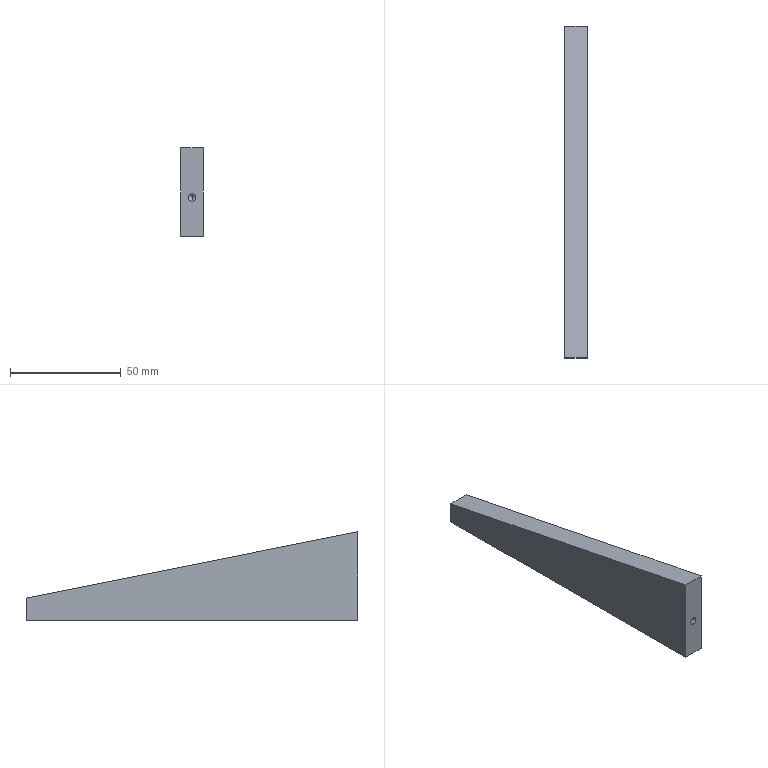Part | SolidWorks | features HoleWzd 2, Chamfer 1, Extrusion 1 | 1 solid | 22 faces | box 10 x 150 x 40 mm | volume 37104 mm3 | cylinder 8 | cone 8 | plane 6 | commonest cylinder face diameters 3.3 x8
STEP:
#1=CARTESIAN_POINT('',(0.,-60.,19.15));
#2=VERTEX_POINT('',#1);
#3=CARTESIAN_POINT('',(0.,-60.,15.85));
#4=VERTEX_POINT('',#3);
#5=CARTESIAN_POINT('',(0.,-60.,17.5));
#6=DIRECTION('',(0.,-1.,0.));
#7=DIRECTION('',(0.,0.,-1.));
#8=AXIS2_PLACEMENT_3D('',#5,#6,#7);
#9=CIRCLE('',#8,1.65);
#10=EDGE_CURVE('',#2,#4,#9,.T.);
#11=ORIENTED_EDGE('',*,*,#10,.F.);
#12=CARTESIAN_POINT('',(0.,-75.,19.15));
#13=VERTEX_POINT('',#12);
#14=CARTESIAN_POINT('',(0.,-75.,19.15));
#15=DIRECTION('',(0.,-1.,0.));
#16=VECTOR('',#15,1000.);
#17=LINE('',#14,#16);
#18=EDGE_CURVE('',#2,#13,#17,.T.);
#19=ORIENTED_EDGE('',*,*,#18,.T.);
#20=CARTESIAN_POINT('',(0.,-75.,15.85));
#21=VERTEX_POINT('',#20);
#22=CARTESIAN_POINT('',(0.,-75.,17.5));
#23=DIRECTION('',(0.,-1.,0.));
#24=DIRECTION('',(0.,0.,-1.));
#25=AXIS2_PLACEMENT_3D('',#22,#23,#24);
#26=CIRCLE('',#25,1.65);
#27=EDGE_CURVE('',#13,#21,#26,.T.);
#28=ORIENTED_EDGE('',*,*,#27,.T.);
#29=CARTESIAN_POINT('',(0.,-75.,15.85));
#30=DIRECTION('',(0.,-1.,0.));
#31=VECTOR('',#30,1000.);
#32=LINE('',#29,#31);
#33=EDGE_CURVE('',#4,#21,#32,.T.);
#34=ORIENTED_EDGE('',*,*,#33,.F.);
#35=EDGE_LOOP('',(#11,#19,#28,#34));
#36=FACE_OUTER_BOUND('',#35,.T.);
#37=CARTESIAN_POINT('',(0.,-75.,17.5));
#38=DIRECTION('',(0.,-1.,0.));
#39=DIRECTION('',(0.,0.,-1.));
#40=AXIS2_PLACEMENT_3D('',#37,#38,#39);
#41=CYLINDRICAL_SURFACE('',#40,1.65);
#42=ADVANCED_FACE('',(#36),#41,.F.);
#43=CARTESIAN_POINT('',(0.,-59.009,17.5));
#44=VERTEX_POINT('',#43);
#45=CARTESIAN_POINT('',(0.,-60.,15.85));
#46=DIRECTION('',(0.,-0.515,-0.8572));
#47=VECTOR('',#46,1000.);
#48=LINE('',#45,#47);
#49=EDGE_CURVE('',#44,#4,#48,.T.);
#50=ORIENTED_EDGE('',*,*,#49,.F.);
#51=CARTESIAN_POINT('',(0.,-60.,19.15));
#52=DIRECTION('',(0.,-0.515,0.8572));
#53=VECTOR('',#52,1000.);
#54=LINE('',#51,#53);
#55=EDGE_CURVE('',#44,#2,#54,.T.);
#56=ORIENTED_EDGE('',*,*,#55,.T.);
#57=ORIENTED_EDGE('',*,*,#10,.T.);
#58=EDGE_LOOP('',(#50,#56,#57));
#59=FACE_OUTER_BOUND('',#58,.T.);
#60=CARTESIAN_POINT('',(0.,-60.,17.5));
#61=DIRECTION('',(0.,-1.,0.));
#62=DIRECTION('',(0.,0.,-1.));
#63=AXIS2_PLACEMENT_3D('',#60,#61,#62);
#64=CONICAL_SURFACE('',#63,1.65,1.03);
#65=ADVANCED_FACE('',(#59),#64,.F.);
#66=CARTESIAN_POINT('',(1.65,50.,10.));
#67=VERTEX_POINT('',#66);
#68=CARTESIAN_POINT('',(-1.65,50.,10.));
#69=VERTEX_POINT('',#68);
#70=CARTESIAN_POINT('',(0.,50.,10.));
#71=DIRECTION('',(0.,0.,-1.));
#72=DIRECTION('',(-1.,0.,0.));
#73=AXIS2_PLACEMENT_3D('',#70,#71,#72);
#74=CIRCLE('',#73,1.65);
#75=EDGE_CURVE('',#67,#69,#74,.T.);
#76=ORIENTED_EDGE('',*,*,#75,.F.);
#77=CARTESIAN_POINT('',(1.65,50.,0.));
#78=VERTEX_POINT('',#77);
#79=CARTESIAN_POINT('',(1.65,50.,0.));
#80=DIRECTION('',(0.,0.,-1.));
#81=VECTOR('',#80,1000.);
#82=LINE('',#79,#81);
#83=EDGE_CURVE('',#67,#78,#82,.T.);
#84=ORIENTED_EDGE('',*,*,#83,.T.);
#85=CARTESIAN_POINT('',(-1.65,50.,0.));
#86=VERTEX_POINT('',#85);
#87=CARTESIAN_POINT('',(0.,50.,0.));
#88=DIRECTION('',(0.,0.,-1.));
#89=DIRECTION('',(-1.,0.,0.));
#90=AXIS2_PLACEMENT_3D('',#87,#88,#89);
#91=CIRCLE('',#90,1.65);
#92=EDGE_CURVE('',#78,#86,#91,.T.);
#93=ORIENTED_EDGE('',*,*,#92,.T.);
#94=CARTESIAN_POINT('',(-1.65,50.,0.));
#95=DIRECTION('',(0.,0.,-1.));
#96=VECTOR('',#95,1000.);
#97=LINE('',#94,#96);
#98=EDGE_CURVE('',#69,#86,#97,.T.);
#99=ORIENTED_EDGE('',*,*,#98,.F.);
#100=EDGE_LOOP('',(#76,#84,#93,#99));
#101=FACE_OUTER_BOUND('',#100,.T.);
#102=CARTESIAN_POINT('',(0.,50.,0.));
#103=DIRECTION('',(0.,0.,-1.));
#104=DIRECTION('',(-1.,0.,0.));
#105=AXIS2_PLACEMENT_3D('',#102,#103,#104);
#106=CYLINDRICAL_SURFACE('',#105,1.65);
#107=ADVANCED_FACE('',(#101),#106,.F.);
#108=CARTESIAN_POINT('',(0.,50.,10.991));
#109=VERTEX_POINT('',#108);
#110=CARTESIAN_POINT('',(-1.65,50.,10.));
#111=DIRECTION('',(-0.8572,0.,-0.515));
#112=VECTOR('',#111,1000.);
#113=LINE('',#110,#112);
#114=EDGE_CURVE('',#109,#69,#113,.T.);
#115=ORIENTED_EDGE('',*,*,#114,.F.);
#116=CARTESIAN_POINT('',(1.65,50.,10.));
#117=DIRECTION('',(0.8572,0.,-0.515));
#118=VECTOR('',#117,1000.);
#119=LINE('',#116,#118);
#120=EDGE_CURVE('',#109,#67,#119,.T.);
#121=ORIENTED_EDGE('',*,*,#120,.T.);
#122=ORIENTED_EDGE('',*,*,#75,.T.);
#123=EDGE_LOOP('',(#115,#121,#122));
#124=FACE_OUTER_BOUND('',#123,.T.);
#125=CARTESIAN_POINT('',(0.,50.,10.));
#126=DIRECTION('',(0.,0.,-1.));
#127=DIRECTION('',(-1.,0.,0.));
#128=AXIS2_PLACEMENT_3D('',#125,#126,#127);
#129=CONICAL_SURFACE('',#128,1.65,1.03);
#130=ADVANCED_FACE('',(#124),#129,.F.);
#131=CARTESIAN_POINT('',(1.65,0.,10.));
#132=VERTEX_POINT('',#131);
#133=CARTESIAN_POINT('',(-1.65,0.,10.));
#134=VERTEX_POINT('',#133);
#135=CARTESIAN_POINT('',(0.,0.,10.));
#136=DIRECTION('',(0.,0.,-1.));
#137=DIRECTION('',(-1.,0.,0.));
#138=AXIS2_PLACEMENT_3D('',#135,#136,#137);
#139=CIRCLE('',#138,1.65);
#140=EDGE_CURVE('',#132,#134,#139,.T.);
#141=ORIENTED_EDGE('',*,*,#140,.F.);
#142=CARTESIAN_POINT('',(1.65,0.,0.));
#143=VERTEX_POINT('',#142);
#144=CARTESIAN_POINT('',(1.65,0.,0.));
#145=DIRECTION('',(0.,0.,-1.));
#146=VECTOR('',#145,1000.);
#147=LINE('',#144,#146);
#148=EDGE_CURVE('',#132,#143,#147,.T.);
#149=ORIENTED_EDGE('',*,*,#148,.T.);
#150=CARTESIAN_POINT('',(-1.65,0.,0.));
#151=VERTEX_POINT('',#150);
#152=CARTESIAN_POINT('',(0.,0.,0.));
#153=DIRECTION('',(0.,0.,-1.));
#154=DIRECTION('',(-1.,0.,0.));
#155=AXIS2_PLACEMENT_3D('',#152,#153,#154);
#156=CIRCLE('',#155,1.65);
#157=EDGE_CURVE('',#143,#151,#156,.T.);
#158=ORIENTED_EDGE('',*,*,#157,.T.);
#159=CARTESIAN_POINT('',(-1.65,0.,0.));
#160=DIRECTION('',(0.,0.,-1.));
#161=VECTOR('',#160,1000.);
#162=LINE('',#159,#161);
#163=EDGE_CURVE('',#134,#151,#162,.T.);
#164=ORIENTED_EDGE('',*,*,#163,.F.);
#165=EDGE_LOOP('',(#141,#149,#158,#164));
#166=FACE_OUTER_BOUND('',#165,.T.);
#167=CARTESIAN_POINT('',(0.,0.,0.));
#168=DIRECTION('',(0.,0.,-1.));
#169=DIRECTION('',(-1.,0.,0.));
#170=AXIS2_PLACEMENT_3D('',#167,#168,#169);
#171=CYLINDRICAL_SURFACE('',#170,1.65);
#172=ADVANCED_FACE('',(#166),#171,.F.);
#173=CARTESIAN_POINT('',(0.,0.,10.991));
#174=VERTEX_POINT('',#173);
#175=CARTESIAN_POINT('',(-1.65,0.,10.));
#176=DIRECTION('',(-0.8572,0.,-0.515));
#177=VECTOR('',#176,1000.);
#178=LINE('',#175,#177);
#179=EDGE_CURVE('',#174,#134,#178,.T.);
#180=ORIENTED_EDGE('',*,*,#179,.F.);
#181=CARTESIAN_POINT('',(1.65,0.,10.));
#182=DIRECTION('',(0.8572,0.,-0.515));
#183=VECTOR('',#182,1000.);
#184=LINE('',#181,#183);
#185=EDGE_CURVE('',#174,#132,#184,.T.);
#186=ORIENTED_EDGE('',*,*,#185,.T.);
#187=ORIENTED_EDGE('',*,*,#140,.T.);
#188=EDGE_LOOP('',(#180,#186,#187));
#189=FACE_OUTER_BOUND('',#188,.T.);
#190=CARTESIAN_POINT('',(0.,0.,10.));
#191=DIRECTION('',(0.,0.,-1.));
#192=DIRECTION('',(-1.,0.,0.));
#193=AXIS2_PLACEMENT_3D('',#190,#191,#192);
#194=CONICAL_SURFACE('',#193,1.65,1.03);
#195=ADVANCED_FACE('',(#189),#194,.F.);
#196=CARTESIAN_POINT('',(1.65,-50.,10.));
#197=VERTEX_POINT('',#196);
#198=CARTESIAN_POINT('',(-1.65,-50.,10.));
#199=VERTEX_POINT('',#198);
#200=CARTESIAN_POINT('',(0.,-50.,10.));
#201=DIRECTION('',(0.,0.,-1.));
#202=DIRECTION('',(-1.,0.,0.));
#203=AXIS2_PLACEMENT_3D('',#200,#201,#202);
#204=CIRCLE('',#203,1.65);
#205=EDGE_CURVE('',#197,#199,#204,.T.);
#206=ORIENTED_EDGE('',*,*,#205,.F.);
#207=CARTESIAN_POINT('',(1.65,-50.,0.));
#208=VERTEX_POINT('',#207);
#209=CARTESIAN_POINT('',(1.65,-50.,0.));
#210=DIRECTION('',(0.,0.,-1.));
#211=VECTOR('',#210,1000.);
#212=LINE('',#209,#211);
#213=EDGE_CURVE('',#197,#208,#212,.T.);
#214=ORIENTED_EDGE('',*,*,#213,.T.);
#215=CARTESIAN_POINT('',(-1.65,-50.,0.));
#216=VERTEX_POINT('',#215);
#217=CARTESIAN_POINT('',(0.,-50.,0.));
#218=DIRECTION('',(0.,0.,-1.));
#219=DIRECTION('',(-1.,0.,0.));
#220=AXIS2_PLACEMENT_3D('',#217,#218,#219);
#221=CIRCLE('',#220,1.65);
#222=EDGE_CURVE('',#208,#216,#221,.T.);
#223=ORIENTED_EDGE('',*,*,#222,.T.);
#224=CARTESIAN_POINT('',(-1.65,-50.,0.));
#225=DIRECTION('',(0.,0.,-1.));
#226=VECTOR('',#225,1000.);
#227=LINE('',#224,#226);
#228=EDGE_CURVE('',#199,#216,#227,.T.);
#229=ORIENTED_EDGE('',*,*,#228,.F.);
#230=EDGE_LOOP('',(#206,#214,#223,#229));
#231=FACE_OUTER_BOUND('',#230,.T.);
#232=CARTESIAN_POINT('',(0.,-50.,0.));
#233=DIRECTION('',(0.,0.,-1.));
#234=DIRECTION('',(-1.,0.,0.));
#235=AXIS2_PLACEMENT_3D('',#232,#233,#234);
#236=CYLINDRICAL_SURFACE('',#235,1.65);
#237=ADVANCED_FACE('',(#231),#236,.F.);
#238=CARTESIAN_POINT('',(0.,-50.,10.991));
#239=VERTEX_POINT('',#238);
#240=CARTESIAN_POINT('',(-1.65,-50.,10.));
#241=DIRECTION('',(-0.8572,0.,-0.515));
#242=VECTOR('',#241,1000.);
#243=LINE('',#240,#242);
#244=EDGE_CURVE('',#239,#199,#243,.T.);
#245=ORIENTED_EDGE('',*,*,#244,.F.);
#246=CARTESIAN_POINT('',(1.65,-50.,10.));
#247=DIRECTION('',(0.8572,0.,-0.515));
#248=VECTOR('',#247,1000.);
#249=LINE('',#246,#248);
#250=EDGE_CURVE('',#239,#197,#249,.T.);
#251=ORIENTED_EDGE('',*,*,#250,.T.);
#252=ORIENTED_EDGE('',*,*,#205,.T.);
#253=EDGE_LOOP('',(#245,#251,#252));
#254=FACE_OUTER_BOUND('',#253,.T.);
#255=CARTESIAN_POINT('',(0.,-50.,10.));
#256=DIRECTION('',(0.,0.,-1.));
#257=DIRECTION('',(-1.,0.,0.));
#258=AXIS2_PLACEMENT_3D('',#255,#256,#257);
#259=CONICAL_SURFACE('',#258,1.65,1.03);
#260=ADVANCED_FACE('',(#254),#259,.F.);
#261=CARTESIAN_POINT('',(5.,75.,10.));
#262=VERTEX_POINT('',#261);
#263=CARTESIAN_POINT('',(5.,75.,0.));
#264=VERTEX_POINT('',#263);
#265=CARTESIAN_POINT('',(5.,75.,40.));
#266=DIRECTION('',(0.,0.,-1.));
#267=VECTOR('',#266,1000.);
#268=LINE('',#265,#267);
#269=EDGE_CURVE('',#262,#264,#268,.T.);
#270=ORIENTED_EDGE('',*,*,#269,.F.);
#271=CARTESIAN_POINT('',(5.,-75.,40.));
#272=VERTEX_POINT('',#271);
#273=CARTESIAN_POINT('',(5.,-75.,40.));
#274=DIRECTION('',(0.,-0.9806,0.1961));
#275=VECTOR('',#274,1000.);
#276=LINE('',#273,#275);
#277=EDGE_CURVE('',#262,#272,#276,.T.);
#278=ORIENTED_EDGE('',*,*,#277,.T.);
#279=CARTESIAN_POINT('',(5.,-75.,0.));
#280=VERTEX_POINT('',#279);
#281=CARTESIAN_POINT('',(5.,-75.,40.));
#282=DIRECTION('',(0.,0.,-1.));
#283=VECTOR('',#282,1000.);
#284=LINE('',#281,#283);
#285=EDGE_CURVE('',#272,#280,#284,.T.);
#286=ORIENTED_EDGE('',*,*,#285,.T.);
#287=CARTESIAN_POINT('',(5.,75.,0.));
#288=DIRECTION('',(0.,1.,0.));
#289=VECTOR('',#288,1000.);
#290=LINE('',#287,#289);
#291=EDGE_CURVE('',#280,#264,#290,.T.);
#292=ORIENTED_EDGE('',*,*,#291,.T.);
#293=EDGE_LOOP('',(#270,#278,#286,#292));
#294=FACE_OUTER_BOUND('',#293,.T.);
#295=CARTESIAN_POINT('',(5.,75.,40.));
#296=DIRECTION('',(-1.,0.,0.));
#297=DIRECTION('',(0.,-1.,0.));
#298=AXIS2_PLACEMENT_3D('',#295,#296,#297);
#299=PLANE('',#298);
#300=ADVANCED_FACE('',(#294),#299,.F.);
#301=CARTESIAN_POINT('',(-5.,75.,10.));
#302=VERTEX_POINT('',#301);
#303=CARTESIAN_POINT('',(-5.,75.,0.));
#304=VERTEX_POINT('',#303);
#305=CARTESIAN_POINT('',(-5.,75.,40.));
#306=DIRECTION('',(0.,0.,-1.));
#307=VECTOR('',#306,1000.);
#308=LINE('',#305,#307);
#309=EDGE_CURVE('',#302,#304,#308,.T.);
#310=ORIENTED_EDGE('',*,*,#309,.F.);
#311=CARTESIAN_POINT('',(5.,75.,10.));
#312=DIRECTION('',(1.,0.,0.));
#313=VECTOR('',#312,1000.);
#314=LINE('',#311,#313);
#315=EDGE_CURVE('',#302,#262,#314,.T.);
#316=ORIENTED_EDGE('',*,*,#315,.T.);
#317=ORIENTED_EDGE('',*,*,#269,.T.);
#318=CARTESIAN_POINT('',(-5.,75.,0.));
#319=DIRECTION('',(-1.,0.,0.));
#320=VECTOR('',#319,1000.);
#321=LINE('',#318,#320);
#322=EDGE_CURVE('',#264,#304,#321,.T.);
#323=ORIENTED_EDGE('',*,*,#322,.T.);
#324=EDGE_LOOP('',(#310,#316,#317,#323));
#325=FACE_OUTER_BOUND('',#324,.T.);
#326=CARTESIAN_POINT('',(-5.,75.,40.));
#327=DIRECTION('',(0.,-1.,0.));
#328=DIRECTION('',(0.,0.,-1.));
#329=AXIS2_PLACEMENT_3D('',#326,#327,#328);
#330=PLANE('',#329);
#331=ADVANCED_FACE('',(#325),#330,.F.);
#332=CARTESIAN_POINT('',(-5.,-75.,40.));
#333=VERTEX_POINT('',#332);
#334=CARTESIAN_POINT('',(-5.,-75.,0.));
#335=VERTEX_POINT('',#334);
#336=CARTESIAN_POINT('',(-5.,-75.,40.));
#337=DIRECTION('',(0.,0.,-1.));
#338=VECTOR('',#337,1000.);
#339=LINE('',#336,#338);
#340=EDGE_CURVE('',#333,#335,#339,.T.);
#341=ORIENTED_EDGE('',*,*,#340,.F.);
#342=CARTESIAN_POINT('',(-5.,-75.,40.));
#343=DIRECTION('',(0.,0.9806,-0.1961));
#344=VECTOR('',#343,1000.);
#345=LINE('',#342,#344);
#346=EDGE_CURVE('',#333,#302,#345,.T.);
#347=ORIENTED_EDGE('',*,*,#346,.T.);
#348=ORIENTED_EDGE('',*,*,#309,.T.);
#349=CARTESIAN_POINT('',(-5.,75.,0.));
#350=DIRECTION('',(0.,-1.,0.));
#351=VECTOR('',#350,1000.);
#352=LINE('',#349,#351);
#353=EDGE_CURVE('',#304,#335,#352,.T.);
#354=ORIENTED_EDGE('',*,*,#353,.T.);
#355=EDGE_LOOP('',(#341,#347,#348,#354));
#356=FACE_OUTER_BOUND('',#355,.T.);
#357=CARTESIAN_POINT('',(-5.,75.,40.));
#358=DIRECTION('',(1.,0.,0.));
#359=DIRECTION('',(0.,1.,0.));
#360=AXIS2_PLACEMENT_3D('',#357,#358,#359);
#361=PLANE('',#360);
#362=ADVANCED_FACE('',(#356),#361,.F.);
#363=CARTESIAN_POINT('',(0.,-75.,17.5));
#364=DIRECTION('',(0.,-1.,0.));
#365=DIRECTION('',(0.,0.,-1.));
#366=AXIS2_PLACEMENT_3D('',#363,#364,#365);
#367=CIRCLE('',#366,1.65);
#368=EDGE_CURVE('',#21,#13,#367,.T.);
#369=ORIENTED_EDGE('',*,*,#368,.F.);
#370=ORIENTED_EDGE('',*,*,#27,.F.);
#371=EDGE_LOOP('',(#369,#370));
#372=FACE_BOUND('',#371,.T.);
#373=CARTESIAN_POINT('',(-5.,-75.,0.));
#374=DIRECTION('',(1.,0.,0.));
#375=VECTOR('',#374,1000.);
#376=LINE('',#373,#375);
#377=EDGE_CURVE('',#335,#280,#376,.T.);
#378=ORIENTED_EDGE('',*,*,#377,.T.);
#379=ORIENTED_EDGE('',*,*,#285,.F.);
#380=CARTESIAN_POINT('',(-5.,-75.,40.));
#381=DIRECTION('',(1.,0.,0.));
#382=VECTOR('',#381,1000.);
#383=LINE('',#380,#382);
#384=EDGE_CURVE('',#333,#272,#383,.T.);
#385=ORIENTED_EDGE('',*,*,#384,.F.);
#386=ORIENTED_EDGE('',*,*,#340,.T.);
#387=EDGE_LOOP('',(#378,#379,#385,#386));
#388=FACE_OUTER_BOUND('',#387,.T.);
#389=CARTESIAN_POINT('',(-5.,-75.,40.));
#390=DIRECTION('',(0.,1.,0.));
#391=DIRECTION('',(0.,0.,1.));
#392=AXIS2_PLACEMENT_3D('',#389,#390,#391);
#393=PLANE('',#392);
#394=ADVANCED_FACE('',(#372,#388),#393,.F.);
#395=CARTESIAN_POINT('',(0.,50.,0.));
#396=DIRECTION('',(0.,0.,-1.));
#397=DIRECTION('',(-1.,0.,0.));
#398=AXIS2_PLACEMENT_3D('',#395,#396,#397);
#399=CIRCLE('',#398,1.65);
#400=EDGE_CURVE('',#86,#78,#399,.T.);
#401=ORIENTED_EDGE('',*,*,#400,.F.);
#402=ORIENTED_EDGE('',*,*,#92,.F.);
#403=EDGE_LOOP('',(#401,#402));
#404=FACE_BOUND('',#403,.T.);
#405=CARTESIAN_POINT('',(0.,0.,0.));
#406=DIRECTION('',(0.,0.,-1.));
#407=DIRECTION('',(-1.,0.,0.));
#408=AXIS2_PLACEMENT_3D('',#405,#406,#407);
#409=CIRCLE('',#408,1.65);
#410=EDGE_CURVE('',#151,#143,#409,.T.);
#411=ORIENTED_EDGE('',*,*,#410,.F.);
#412=ORIENTED_EDGE('',*,*,#157,.F.);
#413=EDGE_LOOP('',(#411,#412));
#414=FACE_BOUND('',#413,.T.);
#415=CARTESIAN_POINT('',(0.,-50.,0.));
#416=DIRECTION('',(0.,0.,-1.));
#417=DIRECTION('',(-1.,0.,0.));
#418=AXIS2_PLACEMENT_3D('',#415,#416,#417);
#419=CIRCLE('',#418,1.65);
#420=EDGE_CURVE('',#216,#208,#419,.T.);
#421=ORIENTED_EDGE('',*,*,#420,.F.);
#422=ORIENTED_EDGE('',*,*,#222,.F.);
#423=EDGE_LOOP('',(#421,#422));
#424=FACE_BOUND('',#423,.T.);
#425=ORIENTED_EDGE('',*,*,#291,.F.);
#426=ORIENTED_EDGE('',*,*,#377,.F.);
#427=ORIENTED_EDGE('',*,*,#353,.F.);
#428=ORIENTED_EDGE('',*,*,#322,.F.);
#429=EDGE_LOOP('',(#425,#426,#427,#428));
#430=FACE_OUTER_BOUND('',#429,.T.);
#431=CARTESIAN_POINT('',(0.,0.,0.));
#432=DIRECTION('',(0.,0.,1.));
#433=DIRECTION('',(1.,0.,0.));
#434=AXIS2_PLACEMENT_3D('',#431,#432,#433);
#435=PLANE('',#434);
#436=ADVANCED_FACE('',(#404,#414,#424,#430),#435,.F.);
#437=ORIENTED_EDGE('',*,*,#250,.F.);
#438=ORIENTED_EDGE('',*,*,#244,.T.);
#439=CARTESIAN_POINT('',(0.,-50.,10.));
#440=DIRECTION('',(0.,0.,-1.));
#441=DIRECTION('',(-1.,0.,0.));
#442=AXIS2_PLACEMENT_3D('',#439,#440,#441);
#443=CIRCLE('',#442,1.65);
#444=EDGE_CURVE('',#199,#197,#443,.T.);
#445=ORIENTED_EDGE('',*,*,#444,.T.);
#446=EDGE_LOOP('',(#437,#438,#445));
#447=FACE_OUTER_BOUND('',#446,.T.);
#448=CARTESIAN_POINT('',(0.,-50.,10.));
#449=DIRECTION('',(0.,0.,-1.));
#450=DIRECTION('',(-1.,0.,0.));
#451=AXIS2_PLACEMENT_3D('',#448,#449,#450);
#452=CONICAL_SURFACE('',#451,1.65,1.03);
#453=ADVANCED_FACE('',(#447),#452,.F.);
#454=ORIENTED_EDGE('',*,*,#213,.F.);
#455=ORIENTED_EDGE('',*,*,#444,.F.);
#456=ORIENTED_EDGE('',*,*,#228,.T.);
#457=ORIENTED_EDGE('',*,*,#420,.T.);
#458=EDGE_LOOP('',(#454,#455,#456,#457));
#459=FACE_OUTER_BOUND('',#458,.T.);
#460=CARTESIAN_POINT('',(0.,-50.,0.));
#461=DIRECTION('',(0.,0.,-1.));
#462=DIRECTION('',(-1.,0.,0.));
#463=AXIS2_PLACEMENT_3D('',#460,#461,#462);
#464=CYLINDRICAL_SURFACE('',#463,1.65);
#465=ADVANCED_FACE('',(#459),#464,.F.);
#466=ORIENTED_EDGE('',*,*,#185,.F.);
#467=ORIENTED_EDGE('',*,*,#179,.T.);
#468=CARTESIAN_POINT('',(0.,0.,10.));
#469=DIRECTION('',(0.,0.,-1.));
#470=DIRECTION('',(-1.,0.,0.));
#471=AXIS2_PLACEMENT_3D('',#468,#469,#470);
#472=CIRCLE('',#471,1.65);
#473=EDGE_CURVE('',#134,#132,#472,.T.);
#474=ORIENTED_EDGE('',*,*,#473,.T.);
#475=EDGE_LOOP('',(#466,#467,#474));
#476=FACE_OUTER_BOUND('',#475,.T.);
#477=CARTESIAN_POINT('',(0.,0.,10.));
#478=DIRECTION('',(0.,0.,-1.));
#479=DIRECTION('',(-1.,0.,0.));
#480=AXIS2_PLACEMENT_3D('',#477,#478,#479);
#481=CONICAL_SURFACE('',#480,1.65,1.03);
#482=ADVANCED_FACE('',(#476),#481,.F.);
#483=ORIENTED_EDGE('',*,*,#148,.F.);
#484=ORIENTED_EDGE('',*,*,#473,.F.);
#485=ORIENTED_EDGE('',*,*,#163,.T.);
#486=ORIENTED_EDGE('',*,*,#410,.T.);
#487=EDGE_LOOP('',(#483,#484,#485,#486));
#488=FACE_OUTER_BOUND('',#487,.T.);
#489=CARTESIAN_POINT('',(0.,0.,0.));
#490=DIRECTION('',(0.,0.,-1.));
#491=DIRECTION('',(-1.,0.,0.));
#492=AXIS2_PLACEMENT_3D('',#489,#490,#491);
#493=CYLINDRICAL_SURFACE('',#492,1.65);
#494=ADVANCED_FACE('',(#488),#493,.F.);
#495=ORIENTED_EDGE('',*,*,#120,.F.);
#496=ORIENTED_EDGE('',*,*,#114,.T.);
#497=CARTESIAN_POINT('',(0.,50.,10.));
#498=DIRECTION('',(0.,0.,-1.));
#499=DIRECTION('',(-1.,0.,0.));
#500=AXIS2_PLACEMENT_3D('',#497,#498,#499);
#501=CIRCLE('',#500,1.65);
#502=EDGE_CURVE('',#69,#67,#501,.T.);
#503=ORIENTED_EDGE('',*,*,#502,.T.);
#504=EDGE_LOOP('',(#495,#496,#503));
#505=FACE_OUTER_BOUND('',#504,.T.);
#506=CARTESIAN_POINT('',(0.,50.,10.));
#507=DIRECTION('',(0.,0.,-1.));
#508=DIRECTION('',(-1.,0.,0.));
#509=AXIS2_PLACEMENT_3D('',#506,#507,#508);
#510=CONICAL_SURFACE('',#509,1.65,1.03);
#511=ADVANCED_FACE('',(#505),#510,.F.);
#512=ORIENTED_EDGE('',*,*,#83,.F.);
#513=ORIENTED_EDGE('',*,*,#502,.F.);
#514=ORIENTED_EDGE('',*,*,#98,.T.);
#515=ORIENTED_EDGE('',*,*,#400,.T.);
#516=EDGE_LOOP('',(#512,#513,#514,#515));
#517=FACE_OUTER_BOUND('',#516,.T.);
#518=CARTESIAN_POINT('',(0.,50.,0.));
#519=DIRECTION('',(0.,0.,-1.));
#520=DIRECTION('',(-1.,0.,0.));
#521=AXIS2_PLACEMENT_3D('',#518,#519,#520);
#522=CYLINDRICAL_SURFACE('',#521,1.65);
#523=ADVANCED_FACE('',(#517),#522,.F.);
#524=ORIENTED_EDGE('',*,*,#55,.F.);
#525=ORIENTED_EDGE('',*,*,#49,.T.);
#526=CARTESIAN_POINT('',(0.,-60.,17.5));
#527=DIRECTION('',(0.,-1.,0.));
#528=DIRECTION('',(0.,0.,-1.));
#529=AXIS2_PLACEMENT_3D('',#526,#527,#528);
#530=CIRCLE('',#529,1.65);
#531=EDGE_CURVE('',#4,#2,#530,.T.);
#532=ORIENTED_EDGE('',*,*,#531,.T.);
#533=EDGE_LOOP('',(#524,#525,#532));
#534=FACE_OUTER_BOUND('',#533,.T.);
#535=CARTESIAN_POINT('',(0.,-60.,17.5));
#536=DIRECTION('',(0.,-1.,0.));
#537=DIRECTION('',(0.,0.,-1.));
#538=AXIS2_PLACEMENT_3D('',#535,#536,#537);
#539=CONICAL_SURFACE('',#538,1.65,1.03);
#540=ADVANCED_FACE('',(#534),#539,.F.);
#541=ORIENTED_EDGE('',*,*,#18,.F.);
#542=ORIENTED_EDGE('',*,*,#531,.F.);
#543=ORIENTED_EDGE('',*,*,#33,.T.);
#544=ORIENTED_EDGE('',*,*,#368,.T.);
#545=EDGE_LOOP('',(#541,#542,#543,#544));
#546=FACE_OUTER_BOUND('',#545,.T.);
#547=CARTESIAN_POINT('',(0.,-75.,17.5));
#548=DIRECTION('',(0.,-1.,0.));
#549=DIRECTION('',(0.,0.,-1.));
#550=AXIS2_PLACEMENT_3D('',#547,#548,#549);
#551=CYLINDRICAL_SURFACE('',#550,1.65);
#552=ADVANCED_FACE('',(#546),#551,.F.);
#553=ORIENTED_EDGE('',*,*,#277,.F.);
#554=ORIENTED_EDGE('',*,*,#315,.F.);
#555=ORIENTED_EDGE('',*,*,#346,.F.);
#556=ORIENTED_EDGE('',*,*,#384,.T.);
#557=EDGE_LOOP('',(#553,#554,#555,#556));
#558=FACE_OUTER_BOUND('',#557,.T.);
#559=CARTESIAN_POINT('',(0.,-75.,40.));
#560=DIRECTION('',(0.,0.1961,0.9806));
#561=DIRECTION('',(1.,0.,0.));
#562=AXIS2_PLACEMENT_3D('',#559,#560,#561);
#563=PLANE('',#562);
#564=ADVANCED_FACE('',(#558),#563,.T.);
#565=CLOSED_SHELL('',(#42,#65,#107,#130,#172,#195,#237,#260,#300,#331,#362,#394,#436,#453,#465,#482,#494,#511,#523,#540,#552,#564));
#566=MANIFOLD_SOLID_BREP('',#565);
#567=CARTESIAN_POINT('',(0.,0.,0.));
#568=DIRECTION('',(0.,0.,1.));
#569=DIRECTION('',(1.,0.,0.));
#570=AXIS2_PLACEMENT_3D('',#567,#568,#569);
#571=(LENGTH_UNIT()NAMED_UNIT(*)SI_UNIT(.MILLI.,.METRE.));
#572=UNCERTAINTY_MEASURE_WITH_UNIT(LENGTH_MEASURE(0.00001),#571,'','');
#573=(NAMED_UNIT(*)PLANE_ANGLE_UNIT()SI_UNIT($,.RADIAN.));
#574=(NAMED_UNIT(*)SI_UNIT($,.STERADIAN.)SOLID_ANGLE_UNIT());
#575=(GEOMETRIC_REPRESENTATION_CONTEXT(3)GLOBAL_UNCERTAINTY_ASSIGNED_CONTEXT((#572))GLOBAL_UNIT_ASSIGNED_CONTEXT((#571,#573,#574))REPRESENTATION_CONTEXT('',''));
#576=ADVANCED_BREP_SHAPE_REPRESENTATION('',(#566,#570),#575);